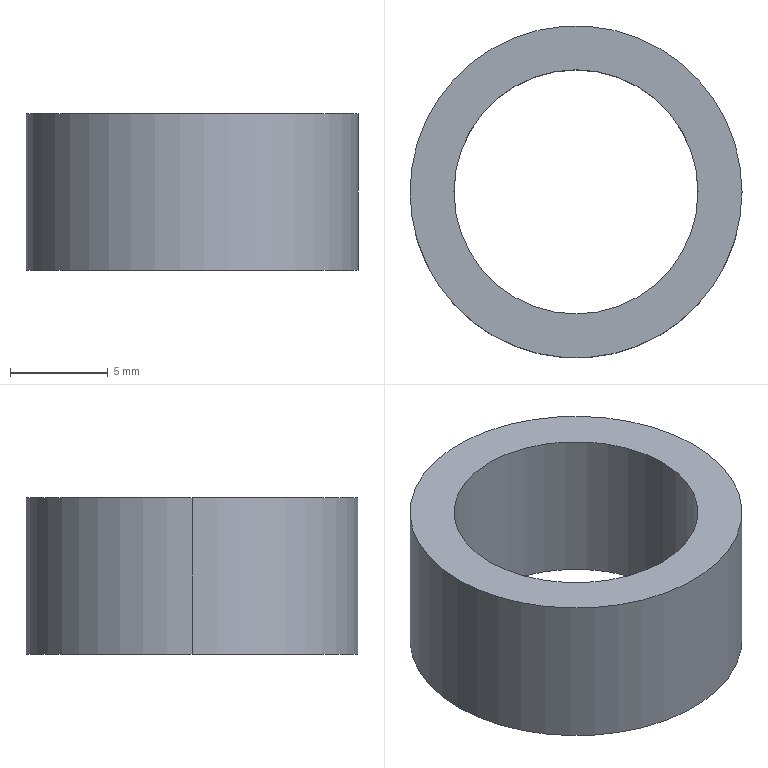Part | SolidWorks | features Extrusion 1 | 1 solid | 6 faces | box 17 x 17 x 8 mm | volume 834.093 mm3 | cylinder 4 | plane 2 | commonest cylinder face diameters 12.5 x2 17 x2
STEP:
#1=CARTESIAN_POINT('',(-6.25,0.,8.));
#2=VERTEX_POINT('',#1);
#3=CARTESIAN_POINT('',(6.25,0.,8.));
#4=VERTEX_POINT('',#3);
#5=CARTESIAN_POINT('',(0.,0.,8.));
#6=DIRECTION('',(0.,0.,1.));
#7=DIRECTION('',(1.,0.,0.));
#8=AXIS2_PLACEMENT_3D('',#5,#6,#7);
#9=CIRCLE('',#8,6.25);
#10=EDGE_CURVE('',#2,#4,#9,.T.);
#11=ORIENTED_EDGE('',*,*,#10,.T.);
#12=CARTESIAN_POINT('',(6.25,0.,0.));
#13=VERTEX_POINT('',#12);
#14=CARTESIAN_POINT('',(6.25,0.,8.));
#15=DIRECTION('',(0.,0.,-1.));
#16=VECTOR('',#15,1000.);
#17=LINE('',#14,#16);
#18=EDGE_CURVE('',#4,#13,#17,.T.);
#19=ORIENTED_EDGE('',*,*,#18,.T.);
#20=CARTESIAN_POINT('',(-6.25,0.,0.));
#21=VERTEX_POINT('',#20);
#22=CARTESIAN_POINT('',(0.,0.,0.));
#23=DIRECTION('',(0.,0.,1.));
#24=DIRECTION('',(1.,0.,0.));
#25=AXIS2_PLACEMENT_3D('',#22,#23,#24);
#26=CIRCLE('',#25,6.25);
#27=EDGE_CURVE('',#21,#13,#26,.T.);
#28=ORIENTED_EDGE('',*,*,#27,.F.);
#29=CARTESIAN_POINT('',(-6.25,0.,8.));
#30=DIRECTION('',(0.,0.,-1.));
#31=VECTOR('',#30,1000.);
#32=LINE('',#29,#31);
#33=EDGE_CURVE('',#2,#21,#32,.T.);
#34=ORIENTED_EDGE('',*,*,#33,.F.);
#35=EDGE_LOOP('',(#11,#19,#28,#34));
#36=FACE_OUTER_BOUND('',#35,.T.);
#37=CARTESIAN_POINT('',(0.,0.,8.));
#38=DIRECTION('',(0.,0.,-1.));
#39=DIRECTION('',(-1.,0.,0.));
#40=AXIS2_PLACEMENT_3D('',#37,#38,#39);
#41=CYLINDRICAL_SURFACE('',#40,6.25);
#42=ADVANCED_FACE('',(#36),#41,.F.);
#43=CARTESIAN_POINT('',(8.5,0.,8.));
#44=VERTEX_POINT('',#43);
#45=CARTESIAN_POINT('',(-8.5,0.,8.));
#46=VERTEX_POINT('',#45);
#47=CARTESIAN_POINT('',(0.,0.,8.));
#48=DIRECTION('',(0.,0.,1.));
#49=DIRECTION('',(1.,0.,0.));
#50=AXIS2_PLACEMENT_3D('',#47,#48,#49);
#51=CIRCLE('',#50,8.5);
#52=EDGE_CURVE('',#44,#46,#51,.T.);
#53=ORIENTED_EDGE('',*,*,#52,.F.);
#54=CARTESIAN_POINT('',(8.5,0.,0.));
#55=VERTEX_POINT('',#54);
#56=CARTESIAN_POINT('',(8.5,0.,8.));
#57=DIRECTION('',(0.,0.,-1.));
#58=VECTOR('',#57,1000.);
#59=LINE('',#56,#58);
#60=EDGE_CURVE('',#44,#55,#59,.T.);
#61=ORIENTED_EDGE('',*,*,#60,.T.);
#62=CARTESIAN_POINT('',(-8.5,0.,0.));
#63=VERTEX_POINT('',#62);
#64=CARTESIAN_POINT('',(0.,0.,0.));
#65=DIRECTION('',(0.,0.,1.));
#66=DIRECTION('',(1.,0.,0.));
#67=AXIS2_PLACEMENT_3D('',#64,#65,#66);
#68=CIRCLE('',#67,8.5);
#69=EDGE_CURVE('',#55,#63,#68,.T.);
#70=ORIENTED_EDGE('',*,*,#69,.T.);
#71=CARTESIAN_POINT('',(-8.5,0.,8.));
#72=DIRECTION('',(0.,0.,-1.));
#73=VECTOR('',#72,1000.);
#74=LINE('',#71,#73);
#75=EDGE_CURVE('',#46,#63,#74,.T.);
#76=ORIENTED_EDGE('',*,*,#75,.F.);
#77=EDGE_LOOP('',(#53,#61,#70,#76));
#78=FACE_OUTER_BOUND('',#77,.T.);
#79=CARTESIAN_POINT('',(0.,0.,8.));
#80=DIRECTION('',(0.,0.,-1.));
#81=DIRECTION('',(-1.,0.,0.));
#82=AXIS2_PLACEMENT_3D('',#79,#80,#81);
#83=CYLINDRICAL_SURFACE('',#82,8.5);
#84=ADVANCED_FACE('',(#78),#83,.T.);
#85=CARTESIAN_POINT('',(0.,0.,8.));
#86=DIRECTION('',(0.,0.,1.));
#87=DIRECTION('',(1.,0.,0.));
#88=AXIS2_PLACEMENT_3D('',#85,#86,#87);
#89=CIRCLE('',#88,8.5);
#90=EDGE_CURVE('',#46,#44,#89,.T.);
#91=ORIENTED_EDGE('',*,*,#90,.T.);
#92=ORIENTED_EDGE('',*,*,#52,.T.);
#93=EDGE_LOOP('',(#91,#92));
#94=FACE_OUTER_BOUND('',#93,.T.);
#95=ORIENTED_EDGE('',*,*,#10,.F.);
#96=CARTESIAN_POINT('',(0.,0.,8.));
#97=DIRECTION('',(0.,0.,1.));
#98=DIRECTION('',(1.,0.,0.));
#99=AXIS2_PLACEMENT_3D('',#96,#97,#98);
#100=CIRCLE('',#99,6.25);
#101=EDGE_CURVE('',#4,#2,#100,.T.);
#102=ORIENTED_EDGE('',*,*,#101,.F.);
#103=EDGE_LOOP('',(#95,#102));
#104=FACE_BOUND('',#103,.T.);
#105=CARTESIAN_POINT('',(0.,0.,8.));
#106=DIRECTION('',(0.,0.,1.));
#107=DIRECTION('',(1.,0.,0.));
#108=AXIS2_PLACEMENT_3D('',#105,#106,#107);
#109=PLANE('',#108);
#110=ADVANCED_FACE('',(#94,#104),#109,.T.);
#111=CARTESIAN_POINT('',(0.,0.,0.));
#112=DIRECTION('',(0.,0.,1.));
#113=DIRECTION('',(1.,0.,0.));
#114=AXIS2_PLACEMENT_3D('',#111,#112,#113);
#115=CIRCLE('',#114,8.5);
#116=EDGE_CURVE('',#63,#55,#115,.T.);
#117=ORIENTED_EDGE('',*,*,#116,.F.);
#118=ORIENTED_EDGE('',*,*,#69,.F.);
#119=EDGE_LOOP('',(#117,#118));
#120=FACE_OUTER_BOUND('',#119,.T.);
#121=ORIENTED_EDGE('',*,*,#27,.T.);
#122=CARTESIAN_POINT('',(0.,0.,0.));
#123=DIRECTION('',(0.,0.,1.));
#124=DIRECTION('',(1.,0.,0.));
#125=AXIS2_PLACEMENT_3D('',#122,#123,#124);
#126=CIRCLE('',#125,6.25);
#127=EDGE_CURVE('',#13,#21,#126,.T.);
#128=ORIENTED_EDGE('',*,*,#127,.T.);
#129=EDGE_LOOP('',(#121,#128));
#130=FACE_BOUND('',#129,.T.);
#131=CARTESIAN_POINT('',(0.,0.,0.));
#132=DIRECTION('',(0.,0.,1.));
#133=DIRECTION('',(1.,0.,0.));
#134=AXIS2_PLACEMENT_3D('',#131,#132,#133);
#135=PLANE('',#134);
#136=ADVANCED_FACE('',(#120,#130),#135,.F.);
#137=ORIENTED_EDGE('',*,*,#60,.F.);
#138=ORIENTED_EDGE('',*,*,#90,.F.);
#139=ORIENTED_EDGE('',*,*,#75,.T.);
#140=ORIENTED_EDGE('',*,*,#116,.T.);
#141=EDGE_LOOP('',(#137,#138,#139,#140));
#142=FACE_OUTER_BOUND('',#141,.T.);
#143=CARTESIAN_POINT('',(0.,0.,8.));
#144=DIRECTION('',(0.,0.,-1.));
#145=DIRECTION('',(-1.,0.,0.));
#146=AXIS2_PLACEMENT_3D('',#143,#144,#145);
#147=CYLINDRICAL_SURFACE('',#146,8.5);
#148=ADVANCED_FACE('',(#142),#147,.T.);
#149=ORIENTED_EDGE('',*,*,#18,.F.);
#150=ORIENTED_EDGE('',*,*,#101,.T.);
#151=ORIENTED_EDGE('',*,*,#33,.T.);
#152=ORIENTED_EDGE('',*,*,#127,.F.);
#153=EDGE_LOOP('',(#149,#150,#151,#152));
#154=FACE_OUTER_BOUND('',#153,.T.);
#155=CARTESIAN_POINT('',(0.,0.,8.));
#156=DIRECTION('',(0.,0.,-1.));
#157=DIRECTION('',(-1.,0.,0.));
#158=AXIS2_PLACEMENT_3D('',#155,#156,#157);
#159=CYLINDRICAL_SURFACE('',#158,6.25);
#160=ADVANCED_FACE('',(#154),#159,.F.);
#161=CLOSED_SHELL('',(#42,#84,#110,#136,#148,#160));
#162=MANIFOLD_SOLID_BREP('',#161);
#163=CARTESIAN_POINT('',(0.,0.,0.));
#164=DIRECTION('',(0.,0.,1.));
#165=DIRECTION('',(1.,0.,0.));
#166=AXIS2_PLACEMENT_3D('',#163,#164,#165);
#167=(LENGTH_UNIT()NAMED_UNIT(*)SI_UNIT(.MILLI.,.METRE.));
#168=UNCERTAINTY_MEASURE_WITH_UNIT(LENGTH_MEASURE(0.00001),#167,'','');
#169=(NAMED_UNIT(*)PLANE_ANGLE_UNIT()SI_UNIT($,.RADIAN.));
#170=(NAMED_UNIT(*)SI_UNIT($,.STERADIAN.)SOLID_ANGLE_UNIT());
#171=(GEOMETRIC_REPRESENTATION_CONTEXT(3)GLOBAL_UNCERTAINTY_ASSIGNED_CONTEXT((#168))GLOBAL_UNIT_ASSIGNED_CONTEXT((#167,#169,#170))REPRESENTATION_CONTEXT('',''));
#172=ADVANCED_BREP_SHAPE_REPRESENTATION('',(#162,#166),#171);